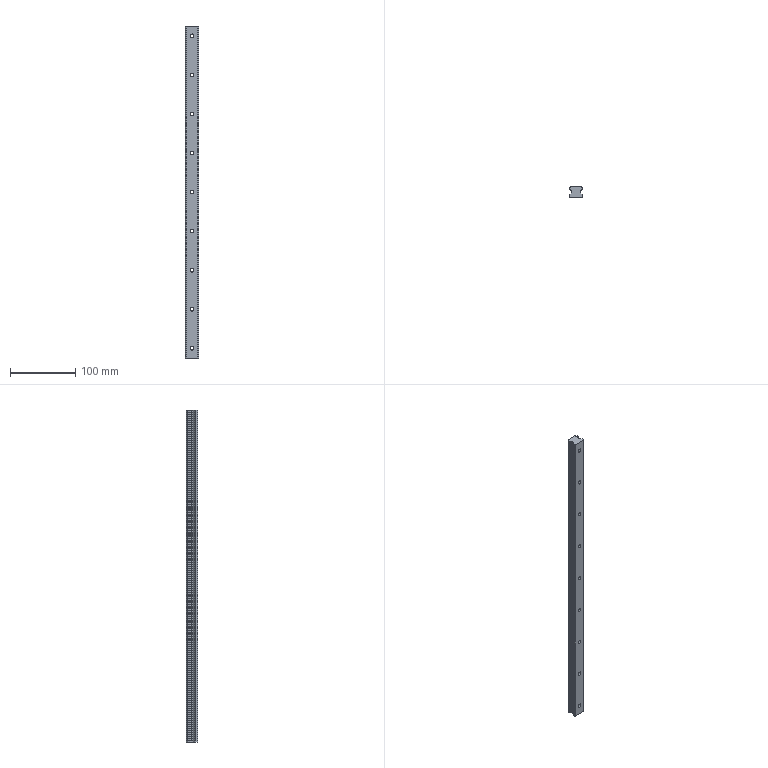Part | SolidWorks | features BaseBody 1, HoleWzd 1, ICE 1, LPattern 1 | 1 solid | 89 faces | box 20 x 17.5 x 510 mm | volume 145503 mm3 | cylinder 58 | plane 31 | commonest cylinder face diameters 1 x12 5.5 x12 10 x12 2 x6 6 x6 9.5 x6